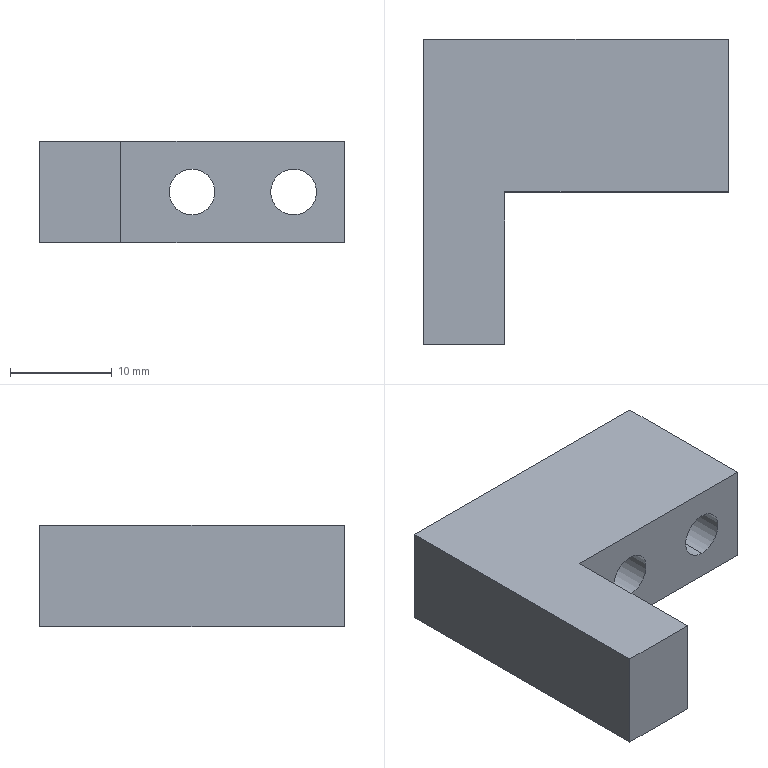Part | STEP file | 227H056244 Stopper_Default | 1 solid | 18 faces | box 30 x 30 x 10 mm | volume 4879 mm3 | plane 10 | cylinder 8 | commonest cylinder face diameters 4.5 x4 8 x4
STEP:
#1=CARTESIAN_POINT('',(0.,0.,0.));
#2=DIRECTION('',(0.,0.,1.));
#3=DIRECTION('',(1.,0.,0.));
#4=AXIS2_PLACEMENT_3D('',#1,#2,#3);
#5=CARTESIAN_POINT('',(10.,10.,4.));
#6=VERTEX_POINT('',#5);
#7=CARTESIAN_POINT('',(10.,15.,4.));
#8=VERTEX_POINT('',#7);
#9=CARTESIAN_POINT('',(10.,15.,4.));
#10=DIRECTION('',(0.,1.,0.));
#11=VECTOR('',#10,1.);
#12=LINE('',#9,#11);
#13=CARTESIAN_POINT('',(10.,15.,0.));
#14=DIRECTION('',(0.,1.,0.));
#15=DIRECTION('',(0.,0.,1.));
#16=AXIS2_PLACEMENT_3D('',#13,#14,#15);
#17=CYLINDRICAL_SURFACE('',#16,4.);
#18=CARTESIAN_POINT('',(6.283,0.));
#19=DIRECTION('',(0.,1.));
#20=VECTOR('',#19,1.);
#21=LINE('',#18,#20);
#22=(GEOMETRIC_REPRESENTATION_CONTEXT(2)PARAMETRIC_REPRESENTATION_CONTEXT()REPRESENTATION_CONTEXT('',''));
#23=DEFINITIONAL_REPRESENTATION('',(#21),#22);
#24=PCURVE('',#17,#23);
#25=CARTESIAN_POINT('',(10.,15.,0.));
#26=DIRECTION('',(0.,1.,0.));
#27=DIRECTION('',(0.,0.,1.));
#28=AXIS2_PLACEMENT_3D('',#25,#26,#27);
#29=CYLINDRICAL_SURFACE('',#28,4.);
#30=CARTESIAN_POINT('',(0.,0.));
#31=DIRECTION('',(0.,1.));
#32=VECTOR('',#31,1.);
#33=LINE('',#30,#32);
#34=(GEOMETRIC_REPRESENTATION_CONTEXT(2)PARAMETRIC_REPRESENTATION_CONTEXT()REPRESENTATION_CONTEXT('',''));
#35=DEFINITIONAL_REPRESENTATION('',(#33),#34);
#36=PCURVE('',#29,#35);
#37=SURFACE_CURVE('',#12,(#24,#36),.PCURVE_S1.);
#38=EDGE_CURVE('',#6,#8,#37,.T.);
#39=ORIENTED_EDGE('',*,*,#38,.T.);
#40=CARTESIAN_POINT('',(10.,15.,-4.));
#41=VERTEX_POINT('',#40);
#42=CARTESIAN_POINT('',(10.,15.,0.));
#43=DIRECTION('',(0.,1.,0.));
#44=DIRECTION('',(0.,0.,1.));
#45=AXIS2_PLACEMENT_3D('',#42,#43,#44);
#46=CIRCLE('',#45,4.);
#47=CARTESIAN_POINT('',(0.,0.));
#48=DIRECTION('',(1.,0.));
#49=VECTOR('',#48,1.);
#50=LINE('',#47,#49);
#51=(GEOMETRIC_REPRESENTATION_CONTEXT(2)PARAMETRIC_REPRESENTATION_CONTEXT()REPRESENTATION_CONTEXT('',''));
#52=DEFINITIONAL_REPRESENTATION('',(#50),#51);
#53=PCURVE('',#17,#52);
#54=CARTESIAN_POINT('',(0.,15.,0.));
#55=DIRECTION('',(0.,1.,0.));
#56=DIRECTION('',(0.,0.,1.));
#57=AXIS2_PLACEMENT_3D('',#54,#55,#56);
#58=PLANE('',#57);
#59=CARTESIAN_POINT('',(0.,10.));
#60=DIRECTION('',(1.,0.));
#61=AXIS2_PLACEMENT_2D('',#59,#60);
#62=CIRCLE('',#61,4.);
#63=(GEOMETRIC_REPRESENTATION_CONTEXT(2)PARAMETRIC_REPRESENTATION_CONTEXT()REPRESENTATION_CONTEXT('',''));
#64=DEFINITIONAL_REPRESENTATION('',(#62),#63);
#65=PCURVE('',#58,#64);
#66=SURFACE_CURVE('',#46,(#53,#65),.PCURVE_S1.);
#67=EDGE_CURVE('',#41,#8,#66,.T.);
#68=ORIENTED_EDGE('',*,*,#67,.F.);
#69=CARTESIAN_POINT('',(10.,10.,-4.));
#70=VERTEX_POINT('',#69);
#71=CARTESIAN_POINT('',(10.,15.,-4.));
#72=DIRECTION('',(0.,1.,0.));
#73=VECTOR('',#72,1.);
#74=LINE('',#71,#73);
#75=CARTESIAN_POINT('',(3.142,0.));
#76=DIRECTION('',(0.,1.));
#77=VECTOR('',#76,1.);
#78=LINE('',#75,#77);
#79=(GEOMETRIC_REPRESENTATION_CONTEXT(2)PARAMETRIC_REPRESENTATION_CONTEXT()REPRESENTATION_CONTEXT('',''));
#80=DEFINITIONAL_REPRESENTATION('',(#78),#79);
#81=PCURVE('',#17,#80);
#82=CARTESIAN_POINT('',(3.142,0.));
#83=DIRECTION('',(0.,1.));
#84=VECTOR('',#83,1.);
#85=LINE('',#82,#84);
#86=(GEOMETRIC_REPRESENTATION_CONTEXT(2)PARAMETRIC_REPRESENTATION_CONTEXT()REPRESENTATION_CONTEXT('',''));
#87=DEFINITIONAL_REPRESENTATION('',(#85),#86);
#88=PCURVE('',#29,#87);
#89=SURFACE_CURVE('',#74,(#81,#88),.PCURVE_S1.);
#90=EDGE_CURVE('',#70,#41,#89,.T.);
#91=ORIENTED_EDGE('',*,*,#90,.F.);
#92=CARTESIAN_POINT('',(10.,10.,0.));
#93=DIRECTION('',(0.,1.,0.));
#94=DIRECTION('',(0.,0.,1.));
#95=AXIS2_PLACEMENT_3D('',#92,#93,#94);
#96=CIRCLE('',#95,4.);
#97=CARTESIAN_POINT('',(0.,-5.));
#98=DIRECTION('',(1.,0.));
#99=VECTOR('',#98,1.);
#100=LINE('',#97,#99);
#101=(GEOMETRIC_REPRESENTATION_CONTEXT(2)PARAMETRIC_REPRESENTATION_CONTEXT()REPRESENTATION_CONTEXT('',''));
#102=DEFINITIONAL_REPRESENTATION('',(#100),#101);
#103=PCURVE('',#17,#102);
#104=CARTESIAN_POINT('',(12.25,10.,0.));
#105=DIRECTION('',(0.,-1.,0.));
#106=DIRECTION('',(0.,0.,-1.));
#107=AXIS2_PLACEMENT_3D('',#104,#105,#106);
#108=PLANE('',#107);
#109=CARTESIAN_POINT('',(-4.,-2.25));
#110=CARTESIAN_POINT('',(-4.,4.678));
#111=CARTESIAN_POINT('',(2.,1.214));
#112=CARTESIAN_POINT('',(8.,-2.25));
#113=CARTESIAN_POINT('',(2.,-5.714));
#114=CARTESIAN_POINT('',(-4.,-9.178));
#115=CARTESIAN_POINT('',(-4.,-2.25));
#116=(BOUNDED_CURVE()B_SPLINE_CURVE(2,(#109,#110,#111,#112,#113,#114,#115),.UNSPECIFIED.,.T.,.F.)B_SPLINE_CURVE_WITH_KNOTS((1,2,2,2,2,1),(-2.094,0.,2.094,4.189,6.283,8.378),.UNSPECIFIED.)CURVE()GEOMETRIC_REPRESENTATION_ITEM()RATIONAL_B_SPLINE_CURVE((1.,0.5,1.,0.5,1.,0.5,1.))REPRESENTATION_ITEM(''));
#117=(GEOMETRIC_REPRESENTATION_CONTEXT(2)PARAMETRIC_REPRESENTATION_CONTEXT()REPRESENTATION_CONTEXT('',''));
#118=DEFINITIONAL_REPRESENTATION('',(#116),#117);
#119=PCURVE('',#108,#118);
#120=SURFACE_CURVE('',#96,(#103,#119),.PCURVE_S1.);
#121=EDGE_CURVE('',#70,#6,#120,.T.);
#122=ORIENTED_EDGE('',*,*,#121,.T.);
#123=EDGE_LOOP('',(#39,#68,#91,#122));
#124=FACE_BOUND('',#123,.F.);
#125=ADVANCED_FACE('',(#124),#17,.F.);
#126=CARTESIAN_POINT('',(10.,0.,2.25));
#127=VERTEX_POINT('',#126);
#128=CARTESIAN_POINT('',(10.,10.,2.25));
#129=VERTEX_POINT('',#128);
#130=CARTESIAN_POINT('',(10.,15.,2.25));
#131=DIRECTION('',(0.,1.,0.));
#132=VECTOR('',#131,1.);
#133=LINE('',#130,#132);
#134=CARTESIAN_POINT('',(10.,15.,0.));
#135=DIRECTION('',(0.,1.,0.));
#136=DIRECTION('',(0.,0.,1.));
#137=AXIS2_PLACEMENT_3D('',#134,#135,#136);
#138=CYLINDRICAL_SURFACE('',#137,2.25);
#139=CARTESIAN_POINT('',(6.283,0.));
#140=DIRECTION('',(0.,1.));
#141=VECTOR('',#140,1.);
#142=LINE('',#139,#141);
#143=(GEOMETRIC_REPRESENTATION_CONTEXT(2)PARAMETRIC_REPRESENTATION_CONTEXT()REPRESENTATION_CONTEXT('',''));
#144=DEFINITIONAL_REPRESENTATION('',(#142),#143);
#145=PCURVE('',#138,#144);
#146=CARTESIAN_POINT('',(10.,15.,0.));
#147=DIRECTION('',(0.,1.,0.));
#148=DIRECTION('',(0.,0.,1.));
#149=AXIS2_PLACEMENT_3D('',#146,#147,#148);
#150=CYLINDRICAL_SURFACE('',#149,2.25);
#151=CARTESIAN_POINT('',(0.,0.));
#152=DIRECTION('',(0.,1.));
#153=VECTOR('',#152,1.);
#154=LINE('',#151,#153);
#155=(GEOMETRIC_REPRESENTATION_CONTEXT(2)PARAMETRIC_REPRESENTATION_CONTEXT()REPRESENTATION_CONTEXT('',''));
#156=DEFINITIONAL_REPRESENTATION('',(#154),#155);
#157=PCURVE('',#150,#156);
#158=SURFACE_CURVE('',#133,(#145,#157),.PCURVE_S1.);
#159=EDGE_CURVE('',#127,#129,#158,.T.);
#160=ORIENTED_EDGE('',*,*,#159,.T.);
#161=CARTESIAN_POINT('',(10.,10.,-2.25));
#162=VERTEX_POINT('',#161);
#163=CARTESIAN_POINT('',(10.,10.,0.));
#164=DIRECTION('',(0.,1.,0.));
#165=DIRECTION('',(0.,0.,1.));
#166=AXIS2_PLACEMENT_3D('',#163,#164,#165);
#167=CIRCLE('',#166,2.25);
#168=CARTESIAN_POINT('',(0.,-5.));
#169=DIRECTION('',(1.,0.));
#170=VECTOR('',#169,1.);
#171=LINE('',#168,#170);
#172=(GEOMETRIC_REPRESENTATION_CONTEXT(2)PARAMETRIC_REPRESENTATION_CONTEXT()REPRESENTATION_CONTEXT('',''));
#173=DEFINITIONAL_REPRESENTATION('',(#171),#172);
#174=PCURVE('',#138,#173);
#175=CARTESIAN_POINT('',(-2.25,-2.25));
#176=CARTESIAN_POINT('',(-2.25,1.647));
#177=CARTESIAN_POINT('',(1.125,-0.3014));
#178=CARTESIAN_POINT('',(4.5,-2.25));
#179=CARTESIAN_POINT('',(1.125,-4.199));
#180=CARTESIAN_POINT('',(-2.25,-6.147));
#181=CARTESIAN_POINT('',(-2.25,-2.25));
#182=(BOUNDED_CURVE()B_SPLINE_CURVE(2,(#175,#176,#177,#178,#179,#180,#181),.UNSPECIFIED.,.T.,.F.)B_SPLINE_CURVE_WITH_KNOTS((1,2,2,2,2,1),(-2.094,0.,2.094,4.189,6.283,8.378),.UNSPECIFIED.)CURVE()GEOMETRIC_REPRESENTATION_ITEM()RATIONAL_B_SPLINE_CURVE((1.,0.5,1.,0.5,1.,0.5,1.))REPRESENTATION_ITEM(''));
#183=(GEOMETRIC_REPRESENTATION_CONTEXT(2)PARAMETRIC_REPRESENTATION_CONTEXT()REPRESENTATION_CONTEXT('',''));
#184=DEFINITIONAL_REPRESENTATION('',(#182),#183);
#185=PCURVE('',#108,#184);
#186=SURFACE_CURVE('',#167,(#174,#185),.PCURVE_S1.);
#187=EDGE_CURVE('',#162,#129,#186,.T.);
#188=ORIENTED_EDGE('',*,*,#187,.F.);
#189=CARTESIAN_POINT('',(10.,0.,-2.25));
#190=VERTEX_POINT('',#189);
#191=CARTESIAN_POINT('',(10.,15.,-2.25));
#192=DIRECTION('',(0.,1.,0.));
#193=VECTOR('',#192,1.);
#194=LINE('',#191,#193);
#195=CARTESIAN_POINT('',(3.142,0.));
#196=DIRECTION('',(0.,1.));
#197=VECTOR('',#196,1.);
#198=LINE('',#195,#197);
#199=(GEOMETRIC_REPRESENTATION_CONTEXT(2)PARAMETRIC_REPRESENTATION_CONTEXT()REPRESENTATION_CONTEXT('',''));
#200=DEFINITIONAL_REPRESENTATION('',(#198),#199);
#201=PCURVE('',#138,#200);
#202=CARTESIAN_POINT('',(3.142,0.));
#203=DIRECTION('',(0.,1.));
#204=VECTOR('',#203,1.);
#205=LINE('',#202,#204);
#206=(GEOMETRIC_REPRESENTATION_CONTEXT(2)PARAMETRIC_REPRESENTATION_CONTEXT()REPRESENTATION_CONTEXT('',''));
#207=DEFINITIONAL_REPRESENTATION('',(#205),#206);
#208=PCURVE('',#150,#207);
#209=SURFACE_CURVE('',#194,(#201,#208),.PCURVE_S1.);
#210=EDGE_CURVE('',#190,#162,#209,.T.);
#211=ORIENTED_EDGE('',*,*,#210,.F.);
#212=CARTESIAN_POINT('',(10.,0.,0.));
#213=DIRECTION('',(0.,1.,0.));
#214=DIRECTION('',(0.,0.,1.));
#215=AXIS2_PLACEMENT_3D('',#212,#213,#214);
#216=CIRCLE('',#215,2.25);
#217=CARTESIAN_POINT('',(0.,-15.));
#218=DIRECTION('',(1.,0.));
#219=VECTOR('',#218,1.);
#220=LINE('',#217,#219);
#221=(GEOMETRIC_REPRESENTATION_CONTEXT(2)PARAMETRIC_REPRESENTATION_CONTEXT()REPRESENTATION_CONTEXT('',''));
#222=DEFINITIONAL_REPRESENTATION('',(#220),#221);
#223=PCURVE('',#138,#222);
#224=CARTESIAN_POINT('',(0.,0.,0.));
#225=DIRECTION('',(0.,1.,0.));
#226=DIRECTION('',(0.,0.,1.));
#227=AXIS2_PLACEMENT_3D('',#224,#225,#226);
#228=PLANE('',#227);
#229=CARTESIAN_POINT('',(0.,10.));
#230=DIRECTION('',(1.,0.));
#231=AXIS2_PLACEMENT_2D('',#229,#230);
#232=CIRCLE('',#231,2.25);
#233=(GEOMETRIC_REPRESENTATION_CONTEXT(2)PARAMETRIC_REPRESENTATION_CONTEXT()REPRESENTATION_CONTEXT('',''));
#234=DEFINITIONAL_REPRESENTATION('',(#232),#233);
#235=PCURVE('',#228,#234);
#236=SURFACE_CURVE('',#216,(#223,#235),.PCURVE_S1.);
#237=EDGE_CURVE('',#190,#127,#236,.T.);
#238=ORIENTED_EDGE('',*,*,#237,.T.);
#239=EDGE_LOOP('',(#160,#188,#211,#238));
#240=FACE_BOUND('',#239,.F.);
#241=ADVANCED_FACE('',(#240),#138,.F.);
#242=CARTESIAN_POINT('',(0.,10.,4.));
#243=VERTEX_POINT('',#242);
#244=CARTESIAN_POINT('',(0.,15.,4.));
#245=VERTEX_POINT('',#244);
#246=CARTESIAN_POINT('',(0.,15.,4.));
#247=DIRECTION('',(0.,1.,0.));
#248=VECTOR('',#247,1.);
#249=LINE('',#246,#248);
#250=CARTESIAN_POINT('',(0.,15.,0.));
#251=DIRECTION('',(0.,1.,0.));
#252=DIRECTION('',(0.,0.,1.));
#253=AXIS2_PLACEMENT_3D('',#250,#251,#252);
#254=CYLINDRICAL_SURFACE('',#253,4.);
#255=CARTESIAN_POINT('',(6.283,0.));
#256=DIRECTION('',(0.,1.));
#257=VECTOR('',#256,1.);
#258=LINE('',#255,#257);
#259=(GEOMETRIC_REPRESENTATION_CONTEXT(2)PARAMETRIC_REPRESENTATION_CONTEXT()REPRESENTATION_CONTEXT('',''));
#260=DEFINITIONAL_REPRESENTATION('',(#258),#259);
#261=PCURVE('',#254,#260);
#262=CARTESIAN_POINT('',(0.,15.,0.));
#263=DIRECTION('',(0.,1.,0.));
#264=DIRECTION('',(0.,0.,1.));
#265=AXIS2_PLACEMENT_3D('',#262,#263,#264);
#266=CYLINDRICAL_SURFACE('',#265,4.);
#267=CARTESIAN_POINT('',(0.,0.));
#268=DIRECTION('',(0.,1.));
#269=VECTOR('',#268,1.);
#270=LINE('',#267,#269);
#271=(GEOMETRIC_REPRESENTATION_CONTEXT(2)PARAMETRIC_REPRESENTATION_CONTEXT()REPRESENTATION_CONTEXT('',''));
#272=DEFINITIONAL_REPRESENTATION('',(#270),#271);
#273=PCURVE('',#266,#272);
#274=SURFACE_CURVE('',#249,(#261,#273),.PCURVE_S1.);
#275=EDGE_CURVE('',#243,#245,#274,.T.);
#276=ORIENTED_EDGE('',*,*,#275,.T.);
#277=CARTESIAN_POINT('',(0.,15.,-4.));
#278=VERTEX_POINT('',#277);
#279=CARTESIAN_POINT('',(0.,15.,0.));
#280=DIRECTION('',(0.,1.,0.));
#281=DIRECTION('',(0.,0.,1.));
#282=AXIS2_PLACEMENT_3D('',#279,#280,#281);
#283=CIRCLE('',#282,4.);
#284=CARTESIAN_POINT('',(0.,0.));
#285=DIRECTION('',(1.,0.));
#286=VECTOR('',#285,1.);
#287=LINE('',#284,#286);
#288=(GEOMETRIC_REPRESENTATION_CONTEXT(2)PARAMETRIC_REPRESENTATION_CONTEXT()REPRESENTATION_CONTEXT('',''));
#289=DEFINITIONAL_REPRESENTATION('',(#287),#288);
#290=PCURVE('',#254,#289);
#291=CARTESIAN_POINT('',(0.,0.));
#292=DIRECTION('',(1.,0.));
#293=AXIS2_PLACEMENT_2D('',#291,#292);
#294=CIRCLE('',#293,4.);
#295=(GEOMETRIC_REPRESENTATION_CONTEXT(2)PARAMETRIC_REPRESENTATION_CONTEXT()REPRESENTATION_CONTEXT('',''));
#296=DEFINITIONAL_REPRESENTATION('',(#294),#295);
#297=PCURVE('',#58,#296);
#298=SURFACE_CURVE('',#283,(#290,#297),.PCURVE_S1.);
#299=EDGE_CURVE('',#278,#245,#298,.T.);
#300=ORIENTED_EDGE('',*,*,#299,.F.);
#301=CARTESIAN_POINT('',(0.,10.,-4.));
#302=VERTEX_POINT('',#301);
#303=CARTESIAN_POINT('',(0.,15.,-4.));
#304=DIRECTION('',(0.,1.,0.));
#305=VECTOR('',#304,1.);
#306=LINE('',#303,#305);
#307=CARTESIAN_POINT('',(3.142,0.));
#308=DIRECTION('',(0.,1.));
#309=VECTOR('',#308,1.);
#310=LINE('',#307,#309);
#311=(GEOMETRIC_REPRESENTATION_CONTEXT(2)PARAMETRIC_REPRESENTATION_CONTEXT()REPRESENTATION_CONTEXT('',''));
#312=DEFINITIONAL_REPRESENTATION('',(#310),#311);
#313=PCURVE('',#254,#312);
#314=CARTESIAN_POINT('',(3.142,0.));
#315=DIRECTION('',(0.,1.));
#316=VECTOR('',#315,1.);
#317=LINE('',#314,#316);
#318=(GEOMETRIC_REPRESENTATION_CONTEXT(2)PARAMETRIC_REPRESENTATION_CONTEXT()REPRESENTATION_CONTEXT('',''));
#319=DEFINITIONAL_REPRESENTATION('',(#317),#318);
#320=PCURVE('',#266,#319);
#321=SURFACE_CURVE('',#306,(#313,#320),.PCURVE_S1.);
#322=EDGE_CURVE('',#302,#278,#321,.T.);
#323=ORIENTED_EDGE('',*,*,#322,.F.);
#324=CARTESIAN_POINT('',(0.,10.,0.));
#325=DIRECTION('',(0.,1.,0.));
#326=DIRECTION('',(0.,0.,1.));
#327=AXIS2_PLACEMENT_3D('',#324,#325,#326);
#328=CIRCLE('',#327,4.);
#329=CARTESIAN_POINT('',(0.,-5.));
#330=DIRECTION('',(1.,0.));
#331=VECTOR('',#330,1.);
#332=LINE('',#329,#331);
#333=(GEOMETRIC_REPRESENTATION_CONTEXT(2)PARAMETRIC_REPRESENTATION_CONTEXT()REPRESENTATION_CONTEXT('',''));
#334=DEFINITIONAL_REPRESENTATION('',(#332),#333);
#335=PCURVE('',#254,#334);
#336=CARTESIAN_POINT('',(2.25,10.,0.));
#337=DIRECTION('',(0.,-1.,0.));
#338=DIRECTION('',(0.,0.,-1.));
#339=AXIS2_PLACEMENT_3D('',#336,#337,#338);
#340=PLANE('',#339);
#341=CARTESIAN_POINT('',(-4.,-2.25));
#342=CARTESIAN_POINT('',(-4.,4.678));
#343=CARTESIAN_POINT('',(2.,1.214));
#344=CARTESIAN_POINT('',(8.,-2.25));
#345=CARTESIAN_POINT('',(2.,-5.714));
#346=CARTESIAN_POINT('',(-4.,-9.178));
#347=CARTESIAN_POINT('',(-4.,-2.25));
#348=(BOUNDED_CURVE()B_SPLINE_CURVE(2,(#341,#342,#343,#344,#345,#346,#347),.UNSPECIFIED.,.T.,.F.)B_SPLINE_CURVE_WITH_KNOTS((1,2,2,2,2,1),(-2.094,0.,2.094,4.189,6.283,8.378),.UNSPECIFIED.)CURVE()GEOMETRIC_REPRESENTATION_ITEM()RATIONAL_B_SPLINE_CURVE((1.,0.5,1.,0.5,1.,0.5,1.))REPRESENTATION_ITEM(''));
#349=(GEOMETRIC_REPRESENTATION_CONTEXT(2)PARAMETRIC_REPRESENTATION_CONTEXT()REPRESENTATION_CONTEXT('',''));
#350=DEFINITIONAL_REPRESENTATION('',(#348),#349);
#351=PCURVE('',#340,#350);
#352=SURFACE_CURVE('',#328,(#335,#351),.PCURVE_S1.);
#353=EDGE_CURVE('',#302,#243,#352,.T.);
#354=ORIENTED_EDGE('',*,*,#353,.T.);
#355=EDGE_LOOP('',(#276,#300,#323,#354));
#356=FACE_BOUND('',#355,.F.);
#357=ADVANCED_FACE('',(#356),#254,.F.);
#358=CARTESIAN_POINT('',(0.,0.,2.25));
#359=VERTEX_POINT('',#358);
#360=CARTESIAN_POINT('',(0.,10.,2.25));
#361=VERTEX_POINT('',#360);
#362=CARTESIAN_POINT('',(0.,15.,2.25));
#363=DIRECTION('',(0.,1.,0.));
#364=VECTOR('',#363,1.);
#365=LINE('',#362,#364);
#366=CARTESIAN_POINT('',(0.,15.,0.));
#367=DIRECTION('',(0.,1.,0.));
#368=DIRECTION('',(0.,0.,1.));
#369=AXIS2_PLACEMENT_3D('',#366,#367,#368);
#370=CYLINDRICAL_SURFACE('',#369,2.25);
#371=CARTESIAN_POINT('',(6.283,0.));
#372=DIRECTION('',(0.,1.));
#373=VECTOR('',#372,1.);
#374=LINE('',#371,#373);
#375=(GEOMETRIC_REPRESENTATION_CONTEXT(2)PARAMETRIC_REPRESENTATION_CONTEXT()REPRESENTATION_CONTEXT('',''));
#376=DEFINITIONAL_REPRESENTATION('',(#374),#375);
#377=PCURVE('',#370,#376);
#378=CARTESIAN_POINT('',(0.,15.,0.));
#379=DIRECTION('',(0.,1.,0.));
#380=DIRECTION('',(0.,0.,1.));
#381=AXIS2_PLACEMENT_3D('',#378,#379,#380);
#382=CYLINDRICAL_SURFACE('',#381,2.25);
#383=CARTESIAN_POINT('',(0.,0.));
#384=DIRECTION('',(0.,1.));
#385=VECTOR('',#384,1.);
#386=LINE('',#383,#385);
#387=(GEOMETRIC_REPRESENTATION_CONTEXT(2)PARAMETRIC_REPRESENTATION_CONTEXT()REPRESENTATION_CONTEXT('',''));
#388=DEFINITIONAL_REPRESENTATION('',(#386),#387);
#389=PCURVE('',#382,#388);
#390=SURFACE_CURVE('',#365,(#377,#389),.PCURVE_S1.);
#391=EDGE_CURVE('',#359,#361,#390,.T.);
#392=ORIENTED_EDGE('',*,*,#391,.T.);
#393=CARTESIAN_POINT('',(0.,10.,-2.25));
#394=VERTEX_POINT('',#393);
#395=CARTESIAN_POINT('',(0.,10.,0.));
#396=DIRECTION('',(0.,1.,0.));
#397=DIRECTION('',(0.,0.,1.));
#398=AXIS2_PLACEMENT_3D('',#395,#396,#397);
#399=CIRCLE('',#398,2.25);
#400=CARTESIAN_POINT('',(0.,-5.));
#401=DIRECTION('',(1.,0.));
#402=VECTOR('',#401,1.);
#403=LINE('',#400,#402);
#404=(GEOMETRIC_REPRESENTATION_CONTEXT(2)PARAMETRIC_REPRESENTATION_CONTEXT()REPRESENTATION_CONTEXT('',''));
#405=DEFINITIONAL_REPRESENTATION('',(#403),#404);
#406=PCURVE('',#370,#405);
#407=CARTESIAN_POINT('',(-2.25,-2.25));
#408=CARTESIAN_POINT('',(-2.25,1.647));
#409=CARTESIAN_POINT('',(1.125,-0.3014));
#410=CARTESIAN_POINT('',(4.5,-2.25));
#411=CARTESIAN_POINT('',(1.125,-4.199));
#412=CARTESIAN_POINT('',(-2.25,-6.147));
#413=CARTESIAN_POINT('',(-2.25,-2.25));
#414=(BOUNDED_CURVE()B_SPLINE_CURVE(2,(#407,#408,#409,#410,#411,#412,#413),.UNSPECIFIED.,.T.,.F.)B_SPLINE_CURVE_WITH_KNOTS((1,2,2,2,2,1),(-2.094,0.,2.094,4.189,6.283,8.378),.UNSPECIFIED.)CURVE()GEOMETRIC_REPRESENTATION_ITEM()RATIONAL_B_SPLINE_CURVE((1.,0.5,1.,0.5,1.,0.5,1.))REPRESENTATION_ITEM(''));
#415=(GEOMETRIC_REPRESENTATION_CONTEXT(2)PARAMETRIC_REPRESENTATION_CONTEXT()REPRESENTATION_CONTEXT('',''));
#416=DEFINITIONAL_REPRESENTATION('',(#414),#415);
#417=PCURVE('',#340,#416);
#418=SURFACE_CURVE('',#399,(#406,#417),.PCURVE_S1.);
#419=EDGE_CURVE('',#394,#361,#418,.T.);
#420=ORIENTED_EDGE('',*,*,#419,.F.);
#421=CARTESIAN_POINT('',(0.,0.,-2.25));
#422=VERTEX_POINT('',#421);
#423=CARTESIAN_POINT('',(0.,15.,-2.25));
#424=DIRECTION('',(0.,1.,0.));
#425=VECTOR('',#424,1.);
#426=LINE('',#423,#425);
#427=CARTESIAN_POINT('',(3.142,0.));
#428=DIRECTION('',(0.,1.));
#429=VECTOR('',#428,1.);
#430=LINE('',#427,#429);
#431=(GEOMETRIC_REPRESENTATION_CONTEXT(2)PARAMETRIC_REPRESENTATION_CONTEXT()REPRESENTATION_CONTEXT('',''));
#432=DEFINITIONAL_REPRESENTATION('',(#430),#431);
#433=PCURVE('',#370,#432);
#434=CARTESIAN_POINT('',(3.142,0.));
#435=DIRECTION('',(0.,1.));
#436=VECTOR('',#435,1.);
#437=LINE('',#434,#436);
#438=(GEOMETRIC_REPRESENTATION_CONTEXT(2)PARAMETRIC_REPRESENTATION_CONTEXT()REPRESENTATION_CONTEXT('',''));
#439=DEFINITIONAL_REPRESENTATION('',(#437),#438);
#440=PCURVE('',#382,#439);
#441=SURFACE_CURVE('',#426,(#433,#440),.PCURVE_S1.);
#442=EDGE_CURVE('',#422,#394,#441,.T.);
#443=ORIENTED_EDGE('',*,*,#442,.F.);
#444=CARTESIAN_POINT('',(0.,0.,0.));
#445=DIRECTION('',(0.,1.,0.));
#446=DIRECTION('',(0.,0.,1.));
#447=AXIS2_PLACEMENT_3D('',#444,#445,#446);
#448=CIRCLE('',#447,2.25);
#449=CARTESIAN_POINT('',(0.,-15.));
#450=DIRECTION('',(1.,0.));
#451=VECTOR('',#450,1.);
#452=LINE('',#449,#451);
#453=(GEOMETRIC_REPRESENTATION_CONTEXT(2)PARAMETRIC_REPRESENTATION_CONTEXT()REPRESENTATION_CONTEXT('',''));
#454=DEFINITIONAL_REPRESENTATION('',(#452),#453);
#455=PCURVE('',#370,#454);
#456=CARTESIAN_POINT('',(0.,0.));
#457=DIRECTION('',(1.,0.));
#458=AXIS2_PLACEMENT_2D('',#456,#457);
#459=CIRCLE('',#458,2.25);
#460=(GEOMETRIC_REPRESENTATION_CONTEXT(2)PARAMETRIC_REPRESENTATION_CONTEXT()REPRESENTATION_CONTEXT('',''));
#461=DEFINITIONAL_REPRESENTATION('',(#459),#460);
#462=PCURVE('',#228,#461);
#463=SURFACE_CURVE('',#448,(#455,#462),.PCURVE_S1.);
#464=EDGE_CURVE('',#422,#359,#463,.T.);
#465=ORIENTED_EDGE('',*,*,#464,.T.);
#466=EDGE_LOOP('',(#392,#420,#443,#465));
#467=FACE_BOUND('',#466,.F.);
#468=ADVANCED_FACE('',(#467),#370,.F.);
#469=CARTESIAN_POINT('',(-15.,15.,-5.));
#470=VERTEX_POINT('',#469);
#471=CARTESIAN_POINT('',(-15.,-15.,-5.));
#472=VERTEX_POINT('',#471);
#473=CARTESIAN_POINT('',(-15.,15.,-5.));
#474=DIRECTION('',(0.,-1.,0.));
#475=VECTOR('',#474,1.);
#476=LINE('',#473,#475);
#477=CARTESIAN_POINT('',(-15.,15.,5.));
#478=DIRECTION('',(1.,0.,0.));
#479=DIRECTION('',(0.,0.,-1.));
#480=AXIS2_PLACEMENT_3D('',#477,#478,#479);
#481=PLANE('',#480);
#482=CARTESIAN_POINT('',(10.,0.));
#483=DIRECTION('',(0.,-1.));
#484=VECTOR('',#483,1.);
#485=LINE('',#482,#484);
#486=(GEOMETRIC_REPRESENTATION_CONTEXT(2)PARAMETRIC_REPRESENTATION_CONTEXT()REPRESENTATION_CONTEXT('',''));
#487=DEFINITIONAL_REPRESENTATION('',(#485),#486);
#488=PCURVE('',#481,#487);
#489=CARTESIAN_POINT('',(15.,15.,-5.));
#490=DIRECTION('',(0.,0.,1.));
#491=DIRECTION('',(1.,0.,0.));
#492=AXIS2_PLACEMENT_3D('',#489,#490,#491);
#493=PLANE('',#492);
#494=CARTESIAN_POINT('',(-30.,0.));
#495=DIRECTION('',(0.,-1.));
#496=VECTOR('',#495,1.);
#497=LINE('',#494,#496);
#498=(GEOMETRIC_REPRESENTATION_CONTEXT(2)PARAMETRIC_REPRESENTATION_CONTEXT()REPRESENTATION_CONTEXT('',''));
#499=DEFINITIONAL_REPRESENTATION('',(#497),#498);
#500=PCURVE('',#493,#499);
#501=SURFACE_CURVE('',#476,(#488,#500),.PCURVE_S1.);
#502=EDGE_CURVE('',#470,#472,#501,.T.);
#503=ORIENTED_EDGE('',*,*,#502,.T.);
#504=CARTESIAN_POINT('',(-15.,-15.,5.));
#505=VERTEX_POINT('',#504);
#506=CARTESIAN_POINT('',(-15.,-15.,22.));
#507=DIRECTION('',(0.,0.,-1.));
#508=VECTOR('',#507,1.);
#509=LINE('',#506,#508);
#510=CARTESIAN_POINT('',(-17.,-30.));
#511=DIRECTION('',(1.,0.));
#512=VECTOR('',#511,1.);
#513=LINE('',#510,#512);
#514=(GEOMETRIC_REPRESENTATION_CONTEXT(2)PARAMETRIC_REPRESENTATION_CONTEXT()REPRESENTATION_CONTEXT('',''));
#515=DEFINITIONAL_REPRESENTATION('',(#513),#514);
#516=PCURVE('',#481,#515);
#517=CARTESIAN_POINT('',(-15.,-15.,22.));
#518=DIRECTION('',(0.,-1.,0.));
#519=DIRECTION('',(0.,0.,-1.));
#520=AXIS2_PLACEMENT_3D('',#517,#518,#519);
#521=PLANE('',#520);
#522=CARTESIAN_POINT('',(0.,0.));
#523=DIRECTION('',(1.,0.));
#524=VECTOR('',#523,1.);
#525=LINE('',#522,#524);
#526=(GEOMETRIC_REPRESENTATION_CONTEXT(2)PARAMETRIC_REPRESENTATION_CONTEXT()REPRESENTATION_CONTEXT('',''));
#527=DEFINITIONAL_REPRESENTATION('',(#525),#526);
#528=PCURVE('',#521,#527);
#529=SURFACE_CURVE('',#509,(#516,#528),.PCURVE_S1.);
#530=EDGE_CURVE('',#505,#472,#529,.T.);
#531=ORIENTED_EDGE('',*,*,#530,.F.);
#532=CARTESIAN_POINT('',(-15.,15.,5.));
#533=VERTEX_POINT('',#532);
#534=CARTESIAN_POINT('',(-15.,15.,5.));
#535=DIRECTION('',(0.,-1.,0.));
#536=VECTOR('',#535,1.);
#537=LINE('',#534,#536);
#538=CARTESIAN_POINT('',(0.,0.));
#539=DIRECTION('',(0.,-1.));
#540=VECTOR('',#539,1.);
#541=LINE('',#538,#540);
#542=(GEOMETRIC_REPRESENTATION_CONTEXT(2)PARAMETRIC_REPRESENTATION_CONTEXT()REPRESENTATION_CONTEXT('',''));
#543=DEFINITIONAL_REPRESENTATION('',(#541),#542);
#544=PCURVE('',#481,#543);
#545=CARTESIAN_POINT('',(15.,15.,5.));
#546=DIRECTION('',(0.,0.,-1.));
#547=DIRECTION('',(-1.,0.,0.));
#548=AXIS2_PLACEMENT_3D('',#545,#546,#547);
#549=PLANE('',#548);
#550=CARTESIAN_POINT('',(30.,0.));
#551=DIRECTION('',(0.,-1.));
#552=VECTOR('',#551,1.);
#553=LINE('',#550,#552);
#554=(GEOMETRIC_REPRESENTATION_CONTEXT(2)PARAMETRIC_REPRESENTATION_CONTEXT()REPRESENTATION_CONTEXT('',''));
#555=DEFINITIONAL_REPRESENTATION('',(#553),#554);
#556=PCURVE('',#549,#555);
#557=SURFACE_CURVE('',#537,(#544,#556),.PCURVE_S1.);
#558=EDGE_CURVE('',#533,#505,#557,.T.);
#559=ORIENTED_EDGE('',*,*,#558,.F.);
#560=CARTESIAN_POINT('',(-15.,15.,5.));
#561=DIRECTION('',(0.,0.,1.));
#562=VECTOR('',#561,1.);
#563=LINE('',#560,#562);
#564=CARTESIAN_POINT('',(0.,0.));
#565=DIRECTION('',(-1.,0.));
#566=VECTOR('',#565,1.);
#567=LINE('',#564,#566);
#568=(GEOMETRIC_REPRESENTATION_CONTEXT(2)PARAMETRIC_REPRESENTATION_CONTEXT()REPRESENTATION_CONTEXT('',''));
#569=DEFINITIONAL_REPRESENTATION('',(#567),#568);
#570=PCURVE('',#481,#569);
#571=CARTESIAN_POINT('',(5.,-15.));
#572=DIRECTION('',(1.,0.));
#573=VECTOR('',#572,1.);
#574=LINE('',#571,#573);
#575=(GEOMETRIC_REPRESENTATION_CONTEXT(2)PARAMETRIC_REPRESENTATION_CONTEXT()REPRESENTATION_CONTEXT('',''));
#576=DEFINITIONAL_REPRESENTATION('',(#574),#575);
#577=PCURVE('',#58,#576);
#578=SURFACE_CURVE('',#563,(#570,#577),.PCURVE_S1.);
#579=EDGE_CURVE('',#470,#533,#578,.T.);
#580=ORIENTED_EDGE('',*,*,#579,.F.);
#581=EDGE_LOOP('',(#503,#531,#559,#580));
#582=FACE_BOUND('',#581,.T.);
#583=ADVANCED_FACE('',(#582),#481,.F.);
#584=ORIENTED_EDGE('',*,*,#558,.T.);
#585=CARTESIAN_POINT('',(-7.,-15.,5.));
#586=VERTEX_POINT('',#585);
#587=CARTESIAN_POINT('',(-15.,-15.,5.));
#588=DIRECTION('',(1.,0.,0.));
#589=VECTOR('',#588,1.);
#590=LINE('',#587,#589);
#591=CARTESIAN_POINT('',(30.,-30.));
#592=DIRECTION('',(-1.,0.));
#593=VECTOR('',#592,1.);
#594=LINE('',#591,#593);
#595=(GEOMETRIC_REPRESENTATION_CONTEXT(2)PARAMETRIC_REPRESENTATION_CONTEXT()REPRESENTATION_CONTEXT('',''));
#596=DEFINITIONAL_REPRESENTATION('',(#594),#595);
#597=PCURVE('',#549,#596);
#598=CARTESIAN_POINT('',(17.,0.));
#599=DIRECTION('',(0.,1.));
#600=VECTOR('',#599,1.);
#601=LINE('',#598,#600);
#602=(GEOMETRIC_REPRESENTATION_CONTEXT(2)PARAMETRIC_REPRESENTATION_CONTEXT()REPRESENTATION_CONTEXT('',''));
#603=DEFINITIONAL_REPRESENTATION('',(#601),#602);
#604=PCURVE('',#521,#603);
#605=SURFACE_CURVE('',#590,(#597,#604),.PCURVE_S1.);
#606=EDGE_CURVE('',#505,#586,#605,.T.);
#607=ORIENTED_EDGE('',*,*,#606,.T.);
#608=CARTESIAN_POINT('',(-7.,0.,5.));
#609=VERTEX_POINT('',#608);
#610=CARTESIAN_POINT('',(-7.,0.,5.));
#611=DIRECTION('',(0.,1.,0.));
#612=VECTOR('',#611,1.);
#613=LINE('',#610,#612);
#614=CARTESIAN_POINT('',(22.,-15.));
#615=DIRECTION('',(0.,1.));
#616=VECTOR('',#615,1.);
#617=LINE('',#614,#616);
#618=(GEOMETRIC_REPRESENTATION_CONTEXT(2)PARAMETRIC_REPRESENTATION_CONTEXT()REPRESENTATION_CONTEXT('',''));
#619=DEFINITIONAL_REPRESENTATION('',(#617),#618);
#620=PCURVE('',#549,#619);
#621=CARTESIAN_POINT('',(-7.,0.,22.));
#622=DIRECTION('',(1.,0.,0.));
#623=DIRECTION('',(0.,1.,0.));
#624=AXIS2_PLACEMENT_3D('',#621,#622,#623);
#625=PLANE('',#624);
#626=CARTESIAN_POINT('',(0.,-17.));
#627=DIRECTION('',(1.,0.));
#628=VECTOR('',#627,1.);
#629=LINE('',#626,#628);
#630=(GEOMETRIC_REPRESENTATION_CONTEXT(2)PARAMETRIC_REPRESENTATION_CONTEXT()REPRESENTATION_CONTEXT('',''));
#631=DEFINITIONAL_REPRESENTATION('',(#629),#630);
#632=PCURVE('',#625,#631);
#633=SURFACE_CURVE('',#613,(#620,#632),.PCURVE_S1.);
#634=EDGE_CURVE('',#586,#609,#633,.T.);
#635=ORIENTED_EDGE('',*,*,#634,.T.);
#636=CARTESIAN_POINT('',(15.,0.,5.));
#637=VERTEX_POINT('',#636);
#638=CARTESIAN_POINT('',(15.,0.,5.));
#639=DIRECTION('',(1.,0.,0.));
#640=VECTOR('',#639,1.);
#641=LINE('',#638,#640);
#642=CARTESIAN_POINT('',(0.,-15.));
#643=DIRECTION('',(-1.,0.));
#644=VECTOR('',#643,1.);
#645=LINE('',#642,#644);
#646=(GEOMETRIC_REPRESENTATION_CONTEXT(2)PARAMETRIC_REPRESENTATION_CONTEXT()REPRESENTATION_CONTEXT('',''));
#647=DEFINITIONAL_REPRESENTATION('',(#645),#646);
#648=PCURVE('',#549,#647);
#649=CARTESIAN_POINT('',(5.,15.));
#650=DIRECTION('',(0.,1.));
#651=VECTOR('',#650,1.);
#652=LINE('',#649,#651);
#653=(GEOMETRIC_REPRESENTATION_CONTEXT(2)PARAMETRIC_REPRESENTATION_CONTEXT()REPRESENTATION_CONTEXT('',''));
#654=DEFINITIONAL_REPRESENTATION('',(#652),#653);
#655=PCURVE('',#228,#654);
#656=SURFACE_CURVE('',#641,(#648,#655),.PCURVE_S1.);
#657=EDGE_CURVE('',#609,#637,#656,.T.);
#658=ORIENTED_EDGE('',*,*,#657,.T.);
#659=CARTESIAN_POINT('',(15.,15.,5.));
#660=VERTEX_POINT('',#659);
#661=CARTESIAN_POINT('',(15.,15.,5.));
#662=DIRECTION('',(0.,-1.,0.));
#663=VECTOR('',#662,1.);
#664=LINE('',#661,#663);
#665=CARTESIAN_POINT('',(0.,0.));
#666=DIRECTION('',(0.,-1.));
#667=VECTOR('',#666,1.);
#668=LINE('',#665,#667);
#669=(GEOMETRIC_REPRESENTATION_CONTEXT(2)PARAMETRIC_REPRESENTATION_CONTEXT()REPRESENTATION_CONTEXT('',''));
#670=DEFINITIONAL_REPRESENTATION('',(#668),#669);
#671=PCURVE('',#549,#670);
#672=CARTESIAN_POINT('',(15.,15.,5.));
#673=DIRECTION('',(-1.,0.,0.));
#674=DIRECTION('',(0.,0.,1.));
#675=AXIS2_PLACEMENT_3D('',#672,#673,#674);
#676=PLANE('',#675);
#677=CARTESIAN_POINT('',(0.,0.));
#678=DIRECTION('',(0.,-1.));
#679=VECTOR('',#678,1.);
#680=LINE('',#677,#679);
#681=(GEOMETRIC_REPRESENTATION_CONTEXT(2)PARAMETRIC_REPRESENTATION_CONTEXT()REPRESENTATION_CONTEXT('',''));
#682=DEFINITIONAL_REPRESENTATION('',(#680),#681);
#683=PCURVE('',#676,#682);
#684=SURFACE_CURVE('',#664,(#671,#683),.PCURVE_S1.);
#685=EDGE_CURVE('',#660,#637,#684,.T.);
#686=ORIENTED_EDGE('',*,*,#685,.F.);
#687=CARTESIAN_POINT('',(15.,15.,5.));
#688=DIRECTION('',(1.,0.,0.));
#689=VECTOR('',#688,1.);
#690=LINE('',#687,#689);
#691=CARTESIAN_POINT('',(0.,0.));
#692=DIRECTION('',(-1.,0.));
#693=VECTOR('',#692,1.);
#694=LINE('',#691,#693);
#695=(GEOMETRIC_REPRESENTATION_CONTEXT(2)PARAMETRIC_REPRESENTATION_CONTEXT()REPRESENTATION_CONTEXT('',''));
#696=DEFINITIONAL_REPRESENTATION('',(#694),#695);
#697=PCURVE('',#549,#696);
#698=CARTESIAN_POINT('',(5.,15.));
#699=DIRECTION('',(0.,1.));
#700=VECTOR('',#699,1.);
#701=LINE('',#698,#700);
#702=(GEOMETRIC_REPRESENTATION_CONTEXT(2)PARAMETRIC_REPRESENTATION_CONTEXT()REPRESENTATION_CONTEXT('',''));
#703=DEFINITIONAL_REPRESENTATION('',(#701),#702);
#704=PCURVE('',#58,#703);
#705=SURFACE_CURVE('',#690,(#697,#704),.PCURVE_S1.);
#706=EDGE_CURVE('',#533,#660,#705,.T.);
#707=ORIENTED_EDGE('',*,*,#706,.F.);
#708=EDGE_LOOP('',(#584,#607,#635,#658,#686,#707));
#709=FACE_BOUND('',#708,.T.);
#710=ADVANCED_FACE('',(#709),#549,.F.);
#711=CARTESIAN_POINT('',(15.,0.,-5.));
#712=VERTEX_POINT('',#711);
#713=CARTESIAN_POINT('',(15.,0.,5.));
#714=DIRECTION('',(0.,0.,-1.));
#715=VECTOR('',#714,1.);
#716=LINE('',#713,#715);
#717=CARTESIAN_POINT('',(0.,-15.));
#718=DIRECTION('',(-1.,0.));
#719=VECTOR('',#718,1.);
#720=LINE('',#717,#719);
#721=(GEOMETRIC_REPRESENTATION_CONTEXT(2)PARAMETRIC_REPRESENTATION_CONTEXT()REPRESENTATION_CONTEXT('',''));
#722=DEFINITIONAL_REPRESENTATION('',(#720),#721);
#723=PCURVE('',#676,#722);
#724=CARTESIAN_POINT('',(5.,15.));
#725=DIRECTION('',(-1.,0.));
#726=VECTOR('',#725,1.);
#727=LINE('',#724,#726);
#728=(GEOMETRIC_REPRESENTATION_CONTEXT(2)PARAMETRIC_REPRESENTATION_CONTEXT()REPRESENTATION_CONTEXT('',''));
#729=DEFINITIONAL_REPRESENTATION('',(#727),#728);
#730=PCURVE('',#228,#729);
#731=SURFACE_CURVE('',#716,(#723,#730),.PCURVE_S1.);
#732=EDGE_CURVE('',#637,#712,#731,.T.);
#733=ORIENTED_EDGE('',*,*,#732,.T.);
#734=CARTESIAN_POINT('',(15.,15.,-5.));
#735=VERTEX_POINT('',#734);
#736=CARTESIAN_POINT('',(15.,15.,-5.));
#737=DIRECTION('',(0.,-1.,0.));
#738=VECTOR('',#737,1.);
#739=LINE('',#736,#738);
#740=CARTESIAN_POINT('',(-10.,0.));
#741=DIRECTION('',(0.,-1.));
#742=VECTOR('',#741,1.);
#743=LINE('',#740,#742);
#744=(GEOMETRIC_REPRESENTATION_CONTEXT(2)PARAMETRIC_REPRESENTATION_CONTEXT()REPRESENTATION_CONTEXT('',''));
#745=DEFINITIONAL_REPRESENTATION('',(#743),#744);
#746=PCURVE('',#676,#745);
#747=CARTESIAN_POINT('',(0.,0.));
#748=DIRECTION('',(0.,-1.));
#749=VECTOR('',#748,1.);
#750=LINE('',#747,#749);
#751=(GEOMETRIC_REPRESENTATION_CONTEXT(2)PARAMETRIC_REPRESENTATION_CONTEXT()REPRESENTATION_CONTEXT('',''));
#752=DEFINITIONAL_REPRESENTATION('',(#750),#751);
#753=PCURVE('',#493,#752);
#754=SURFACE_CURVE('',#739,(#746,#753),.PCURVE_S1.);
#755=EDGE_CURVE('',#735,#712,#754,.T.);
#756=ORIENTED_EDGE('',*,*,#755,.F.);
#757=CARTESIAN_POINT('',(15.,15.,5.));
#758=DIRECTION('',(0.,0.,-1.));
#759=VECTOR('',#758,1.);
#760=LINE('',#757,#759);
#761=CARTESIAN_POINT('',(0.,0.));
#762=DIRECTION('',(-1.,0.));
#763=VECTOR('',#762,1.);
#764=LINE('',#761,#763);
#765=(GEOMETRIC_REPRESENTATION_CONTEXT(2)PARAMETRIC_REPRESENTATION_CONTEXT()REPRESENTATION_CONTEXT('',''));
#766=DEFINITIONAL_REPRESENTATION('',(#764),#765);
#767=PCURVE('',#676,#766);
#768=CARTESIAN_POINT('',(5.,15.));
#769=DIRECTION('',(-1.,0.));
#770=VECTOR('',#769,1.);
#771=LINE('',#768,#770);
#772=(GEOMETRIC_REPRESENTATION_CONTEXT(2)PARAMETRIC_REPRESENTATION_CONTEXT()REPRESENTATION_CONTEXT('',''));
#773=DEFINITIONAL_REPRESENTATION('',(#771),#772);
#774=PCURVE('',#58,#773);
#775=SURFACE_CURVE('',#760,(#767,#774),.PCURVE_S1.);
#776=EDGE_CURVE('',#660,#735,#775,.T.);
#777=ORIENTED_EDGE('',*,*,#776,.F.);
#778=ORIENTED_EDGE('',*,*,#685,.T.);
#779=EDGE_LOOP('',(#733,#756,#777,#778));
#780=FACE_BOUND('',#779,.T.);
#781=ADVANCED_FACE('',(#780),#676,.F.);
#782=CARTESIAN_POINT('',(-7.,0.,-5.));
#783=VERTEX_POINT('',#782);
#784=CARTESIAN_POINT('',(15.,0.,-5.));
#785=DIRECTION('',(-1.,0.,0.));
#786=VECTOR('',#785,1.);
#787=LINE('',#784,#786);
#788=CARTESIAN_POINT('',(0.,-15.));
#789=DIRECTION('',(-1.,0.));
#790=VECTOR('',#789,1.);
#791=LINE('',#788,#790);
#792=(GEOMETRIC_REPRESENTATION_CONTEXT(2)PARAMETRIC_REPRESENTATION_CONTEXT()REPRESENTATION_CONTEXT('',''));
#793=DEFINITIONAL_REPRESENTATION('',(#791),#792);
#794=PCURVE('',#493,#793);
#795=CARTESIAN_POINT('',(-5.,15.));
#796=DIRECTION('',(0.,-1.));
#797=VECTOR('',#796,1.);
#798=LINE('',#795,#797);
#799=(GEOMETRIC_REPRESENTATION_CONTEXT(2)PARAMETRIC_REPRESENTATION_CONTEXT()REPRESENTATION_CONTEXT('',''));
#800=DEFINITIONAL_REPRESENTATION('',(#798),#799);
#801=PCURVE('',#228,#800);
#802=SURFACE_CURVE('',#787,(#794,#801),.PCURVE_S1.);
#803=EDGE_CURVE('',#712,#783,#802,.T.);
#804=ORIENTED_EDGE('',*,*,#803,.T.);
#805=CARTESIAN_POINT('',(-7.,-15.,-5.));
#806=VERTEX_POINT('',#805);
#807=CARTESIAN_POINT('',(-7.,0.,-5.));
#808=DIRECTION('',(0.,-1.,0.));
#809=VECTOR('',#808,1.);
#810=LINE('',#807,#809);
#811=CARTESIAN_POINT('',(-22.,-15.));
#812=DIRECTION('',(0.,-1.));
#813=VECTOR('',#812,1.);
#814=LINE('',#811,#813);
#815=(GEOMETRIC_REPRESENTATION_CONTEXT(2)PARAMETRIC_REPRESENTATION_CONTEXT()REPRESENTATION_CONTEXT('',''));
#816=DEFINITIONAL_REPRESENTATION('',(#814),#815);
#817=PCURVE('',#493,#816);
#818=CARTESIAN_POINT('',(0.,-27.));
#819=DIRECTION('',(-1.,0.));
#820=VECTOR('',#819,1.);
#821=LINE('',#818,#820);
#822=(GEOMETRIC_REPRESENTATION_CONTEXT(2)PARAMETRIC_REPRESENTATION_CONTEXT()REPRESENTATION_CONTEXT('',''));
#823=DEFINITIONAL_REPRESENTATION('',(#821),#822);
#824=PCURVE('',#625,#823);
#825=SURFACE_CURVE('',#810,(#817,#824),.PCURVE_S1.);
#826=EDGE_CURVE('',#783,#806,#825,.T.);
#827=ORIENTED_EDGE('',*,*,#826,.T.);
#828=CARTESIAN_POINT('',(-15.,-15.,-5.));
#829=DIRECTION('',(-1.,0.,0.));
#830=VECTOR('',#829,1.);
#831=LINE('',#828,#830);
#832=CARTESIAN_POINT('',(-30.,-30.));
#833=DIRECTION('',(-1.,0.));
#834=VECTOR('',#833,1.);
#835=LINE('',#832,#834);
#836=(GEOMETRIC_REPRESENTATION_CONTEXT(2)PARAMETRIC_REPRESENTATION_CONTEXT()REPRESENTATION_CONTEXT('',''));
#837=DEFINITIONAL_REPRESENTATION('',(#835),#836);
#838=PCURVE('',#493,#837);
#839=CARTESIAN_POINT('',(27.,0.));
#840=DIRECTION('',(0.,-1.));
#841=VECTOR('',#840,1.);
#842=LINE('',#839,#841);
#843=(GEOMETRIC_REPRESENTATION_CONTEXT(2)PARAMETRIC_REPRESENTATION_CONTEXT()REPRESENTATION_CONTEXT('',''));
#844=DEFINITIONAL_REPRESENTATION('',(#842),#843);
#845=PCURVE('',#521,#844);
#846=SURFACE_CURVE('',#831,(#838,#845),.PCURVE_S1.);
#847=EDGE_CURVE('',#806,#472,#846,.T.);
#848=ORIENTED_EDGE('',*,*,#847,.T.);
#849=ORIENTED_EDGE('',*,*,#502,.F.);
#850=CARTESIAN_POINT('',(15.,15.,-5.));
#851=DIRECTION('',(-1.,0.,0.));
#852=VECTOR('',#851,1.);
#853=LINE('',#850,#852);
#854=CARTESIAN_POINT('',(0.,0.));
#855=DIRECTION('',(-1.,0.));
#856=VECTOR('',#855,1.);
#857=LINE('',#854,#856);
#858=(GEOMETRIC_REPRESENTATION_CONTEXT(2)PARAMETRIC_REPRESENTATION_CONTEXT()REPRESENTATION_CONTEXT('',''));
#859=DEFINITIONAL_REPRESENTATION('',(#857),#858);
#860=PCURVE('',#493,#859);
#861=CARTESIAN_POINT('',(-5.,15.));
#862=DIRECTION('',(0.,-1.));
#863=VECTOR('',#862,1.);
#864=LINE('',#861,#863);
#865=(GEOMETRIC_REPRESENTATION_CONTEXT(2)PARAMETRIC_REPRESENTATION_CONTEXT()REPRESENTATION_CONTEXT('',''));
#866=DEFINITIONAL_REPRESENTATION('',(#864),#865);
#867=PCURVE('',#58,#866);
#868=SURFACE_CURVE('',#853,(#860,#867),.PCURVE_S1.);
#869=EDGE_CURVE('',#735,#470,#868,.T.);
#870=ORIENTED_EDGE('',*,*,#869,.F.);
#871=ORIENTED_EDGE('',*,*,#755,.T.);
#872=EDGE_LOOP('',(#804,#827,#848,#849,#870,#871));
#873=FACE_BOUND('',#872,.T.);
#874=ADVANCED_FACE('',(#873),#493,.F.);
#875=CARTESIAN_POINT('',(10.,15.,0.));
#876=DIRECTION('',(0.,1.,0.));
#877=DIRECTION('',(0.,0.,1.));
#878=AXIS2_PLACEMENT_3D('',#875,#876,#877);
#879=CIRCLE('',#878,4.);
#880=CARTESIAN_POINT('',(0.,10.));
#881=DIRECTION('',(1.,0.));
#882=AXIS2_PLACEMENT_2D('',#880,#881);
#883=CIRCLE('',#882,4.);
#884=(GEOMETRIC_REPRESENTATION_CONTEXT(2)PARAMETRIC_REPRESENTATION_CONTEXT()REPRESENTATION_CONTEXT('',''));
#885=DEFINITIONAL_REPRESENTATION('',(#883),#884);
#886=PCURVE('',#58,#885);
#887=CARTESIAN_POINT('',(0.,0.));
#888=DIRECTION('',(1.,0.));
#889=VECTOR('',#888,1.);
#890=LINE('',#887,#889);
#891=(GEOMETRIC_REPRESENTATION_CONTEXT(2)PARAMETRIC_REPRESENTATION_CONTEXT()REPRESENTATION_CONTEXT('',''));
#892=DEFINITIONAL_REPRESENTATION('',(#890),#891);
#893=PCURVE('',#29,#892);
#894=SURFACE_CURVE('',#879,(#886,#893),.PCURVE_S1.);
#895=EDGE_CURVE('',#8,#41,#894,.T.);
#896=ORIENTED_EDGE('',*,*,#895,.F.);
#897=ORIENTED_EDGE('',*,*,#67,.F.);
#898=EDGE_LOOP('',(#896,#897));
#899=FACE_BOUND('',#898,.T.);
#900=CARTESIAN_POINT('',(0.,15.,0.));
#901=DIRECTION('',(0.,1.,0.));
#902=DIRECTION('',(0.,0.,1.));
#903=AXIS2_PLACEMENT_3D('',#900,#901,#902);
#904=CIRCLE('',#903,4.);
#905=CARTESIAN_POINT('',(0.,0.));
#906=DIRECTION('',(1.,0.));
#907=AXIS2_PLACEMENT_2D('',#905,#906);
#908=CIRCLE('',#907,4.);
#909=(GEOMETRIC_REPRESENTATION_CONTEXT(2)PARAMETRIC_REPRESENTATION_CONTEXT()REPRESENTATION_CONTEXT('',''));
#910=DEFINITIONAL_REPRESENTATION('',(#908),#909);
#911=PCURVE('',#58,#910);
#912=CARTESIAN_POINT('',(0.,0.));
#913=DIRECTION('',(1.,0.));
#914=VECTOR('',#913,1.);
#915=LINE('',#912,#914);
#916=(GEOMETRIC_REPRESENTATION_CONTEXT(2)PARAMETRIC_REPRESENTATION_CONTEXT()REPRESENTATION_CONTEXT('',''));
#917=DEFINITIONAL_REPRESENTATION('',(#915),#916);
#918=PCURVE('',#266,#917);
#919=SURFACE_CURVE('',#904,(#911,#918),.PCURVE_S1.);
#920=EDGE_CURVE('',#245,#278,#919,.T.);
#921=ORIENTED_EDGE('',*,*,#920,.F.);
#922=ORIENTED_EDGE('',*,*,#299,.F.);
#923=EDGE_LOOP('',(#921,#922));
#924=FACE_BOUND('',#923,.T.);
#925=ORIENTED_EDGE('',*,*,#579,.T.);
#926=ORIENTED_EDGE('',*,*,#706,.T.);
#927=ORIENTED_EDGE('',*,*,#776,.T.);
#928=ORIENTED_EDGE('',*,*,#869,.T.);
#929=EDGE_LOOP('',(#925,#926,#927,#928));
#930=FACE_BOUND('',#929,.T.);
#931=ADVANCED_FACE('',(#899,#924,#930),#58,.T.);
#932=CARTESIAN_POINT('',(10.,0.,0.));
#933=DIRECTION('',(0.,1.,0.));
#934=DIRECTION('',(0.,0.,1.));
#935=AXIS2_PLACEMENT_3D('',#932,#933,#934);
#936=CIRCLE('',#935,2.25);
#937=CARTESIAN_POINT('',(0.,10.));
#938=DIRECTION('',(1.,0.));
#939=AXIS2_PLACEMENT_2D('',#937,#938);
#940=CIRCLE('',#939,2.25);
#941=(GEOMETRIC_REPRESENTATION_CONTEXT(2)PARAMETRIC_REPRESENTATION_CONTEXT()REPRESENTATION_CONTEXT('',''));
#942=DEFINITIONAL_REPRESENTATION('',(#940),#941);
#943=PCURVE('',#228,#942);
#944=CARTESIAN_POINT('',(0.,-15.));
#945=DIRECTION('',(1.,0.));
#946=VECTOR('',#945,1.);
#947=LINE('',#944,#946);
#948=(GEOMETRIC_REPRESENTATION_CONTEXT(2)PARAMETRIC_REPRESENTATION_CONTEXT()REPRESENTATION_CONTEXT('',''));
#949=DEFINITIONAL_REPRESENTATION('',(#947),#948);
#950=PCURVE('',#150,#949);
#951=SURFACE_CURVE('',#936,(#943,#950),.PCURVE_S1.);
#952=EDGE_CURVE('',#127,#190,#951,.T.);
#953=ORIENTED_EDGE('',*,*,#952,.T.);
#954=ORIENTED_EDGE('',*,*,#237,.T.);
#955=EDGE_LOOP('',(#953,#954));
#956=FACE_BOUND('',#955,.T.);
#957=CARTESIAN_POINT('',(0.,0.,0.));
#958=DIRECTION('',(0.,1.,0.));
#959=DIRECTION('',(0.,0.,1.));
#960=AXIS2_PLACEMENT_3D('',#957,#958,#959);
#961=CIRCLE('',#960,2.25);
#962=CARTESIAN_POINT('',(0.,0.));
#963=DIRECTION('',(1.,0.));
#964=AXIS2_PLACEMENT_2D('',#962,#963);
#965=CIRCLE('',#964,2.25);
#966=(GEOMETRIC_REPRESENTATION_CONTEXT(2)PARAMETRIC_REPRESENTATION_CONTEXT()REPRESENTATION_CONTEXT('',''));
#967=DEFINITIONAL_REPRESENTATION('',(#965),#966);
#968=PCURVE('',#228,#967);
#969=CARTESIAN_POINT('',(0.,-15.));
#970=DIRECTION('',(1.,0.));
#971=VECTOR('',#970,1.);
#972=LINE('',#969,#971);
#973=(GEOMETRIC_REPRESENTATION_CONTEXT(2)PARAMETRIC_REPRESENTATION_CONTEXT()REPRESENTATION_CONTEXT('',''));
#974=DEFINITIONAL_REPRESENTATION('',(#972),#973);
#975=PCURVE('',#382,#974);
#976=SURFACE_CURVE('',#961,(#968,#975),.PCURVE_S1.);
#977=EDGE_CURVE('',#359,#422,#976,.T.);
#978=ORIENTED_EDGE('',*,*,#977,.T.);
#979=ORIENTED_EDGE('',*,*,#464,.T.);
#980=EDGE_LOOP('',(#978,#979));
#981=FACE_BOUND('',#980,.T.);
#982=ORIENTED_EDGE('',*,*,#657,.F.);
#983=CARTESIAN_POINT('',(-7.,0.,22.));
#984=DIRECTION('',(0.,0.,-1.));
#985=VECTOR('',#984,1.);
#986=LINE('',#983,#985);
#987=CARTESIAN_POINT('',(22.,-7.));
#988=DIRECTION('',(-1.,0.));
#989=VECTOR('',#988,1.);
#990=LINE('',#987,#989);
#991=(GEOMETRIC_REPRESENTATION_CONTEXT(2)PARAMETRIC_REPRESENTATION_CONTEXT()REPRESENTATION_CONTEXT('',''));
#992=DEFINITIONAL_REPRESENTATION('',(#990),#991);
#993=PCURVE('',#228,#992);
#994=CARTESIAN_POINT('',(0.,0.));
#995=DIRECTION('',(0.,-1.));
#996=VECTOR('',#995,1.);
#997=LINE('',#994,#996);
#998=(GEOMETRIC_REPRESENTATION_CONTEXT(2)PARAMETRIC_REPRESENTATION_CONTEXT()REPRESENTATION_CONTEXT('',''));
#999=DEFINITIONAL_REPRESENTATION('',(#997),#998);
#1000=PCURVE('',#625,#999);
#1001=SURFACE_CURVE('',#986,(#993,#1000),.PCURVE_S1.);
#1002=EDGE_CURVE('',#609,#783,#1001,.T.);
#1003=ORIENTED_EDGE('',*,*,#1002,.T.);
#1004=ORIENTED_EDGE('',*,*,#803,.F.);
#1005=ORIENTED_EDGE('',*,*,#732,.F.);
#1006=EDGE_LOOP('',(#982,#1003,#1004,#1005));
#1007=FACE_BOUND('',#1006,.T.);
#1008=ADVANCED_FACE('',(#956,#981,#1007),#228,.F.);
#1009=ORIENTED_EDGE('',*,*,#606,.F.);
#1010=ORIENTED_EDGE('',*,*,#530,.T.);
#1011=ORIENTED_EDGE('',*,*,#847,.F.);
#1012=CARTESIAN_POINT('',(-7.,-15.,22.));
#1013=DIRECTION('',(0.,0.,-1.));
#1014=VECTOR('',#1013,1.);
#1015=LINE('',#1012,#1014);
#1016=CARTESIAN_POINT('',(0.,8.));
#1017=DIRECTION('',(1.,0.));
#1018=VECTOR('',#1017,1.);
#1019=LINE('',#1016,#1018);
#1020=(GEOMETRIC_REPRESENTATION_CONTEXT(2)PARAMETRIC_REPRESENTATION_CONTEXT()REPRESENTATION_CONTEXT('',''));
#1021=DEFINITIONAL_REPRESENTATION('',(#1019),#1020);
#1022=PCURVE('',#521,#1021);
#1023=CARTESIAN_POINT('',(-15.,0.));
#1024=DIRECTION('',(0.,-1.));
#1025=VECTOR('',#1024,1.);
#1026=LINE('',#1023,#1025);
#1027=(GEOMETRIC_REPRESENTATION_CONTEXT(2)PARAMETRIC_REPRESENTATION_CONTEXT()REPRESENTATION_CONTEXT('',''));
#1028=DEFINITIONAL_REPRESENTATION('',(#1026),#1027);
#1029=PCURVE('',#625,#1028);
#1030=SURFACE_CURVE('',#1015,(#1022,#1029),.PCURVE_S1.);
#1031=EDGE_CURVE('',#586,#806,#1030,.T.);
#1032=ORIENTED_EDGE('',*,*,#1031,.F.);
#1033=EDGE_LOOP('',(#1009,#1010,#1011,#1032));
#1034=FACE_BOUND('',#1033,.T.);
#1035=ADVANCED_FACE('',(#1034),#521,.T.);
#1036=ORIENTED_EDGE('',*,*,#634,.F.);
#1037=ORIENTED_EDGE('',*,*,#1031,.T.);
#1038=ORIENTED_EDGE('',*,*,#826,.F.);
#1039=ORIENTED_EDGE('',*,*,#1002,.F.);
#1040=EDGE_LOOP('',(#1036,#1037,#1038,#1039));
#1041=FACE_BOUND('',#1040,.T.);
#1042=ADVANCED_FACE('',(#1041),#625,.T.);
#1043=CARTESIAN_POINT('',(0.,10.,0.));
#1044=DIRECTION('',(0.,1.,0.));
#1045=DIRECTION('',(0.,0.,1.));
#1046=AXIS2_PLACEMENT_3D('',#1043,#1044,#1045);
#1047=CIRCLE('',#1046,2.25);
#1048=CARTESIAN_POINT('',(0.,-5.));
#1049=DIRECTION('',(1.,0.));
#1050=VECTOR('',#1049,1.);
#1051=LINE('',#1048,#1050);
#1052=(GEOMETRIC_REPRESENTATION_CONTEXT(2)PARAMETRIC_REPRESENTATION_CONTEXT()REPRESENTATION_CONTEXT('',''));
#1053=DEFINITIONAL_REPRESENTATION('',(#1051),#1052);
#1054=PCURVE('',#382,#1053);
#1055=CARTESIAN_POINT('',(-2.25,-2.25));
#1056=CARTESIAN_POINT('',(-2.25,1.647));
#1057=CARTESIAN_POINT('',(1.125,-0.3014));
#1058=CARTESIAN_POINT('',(4.5,-2.25));
#1059=CARTESIAN_POINT('',(1.125,-4.199));
#1060=CARTESIAN_POINT('',(-2.25,-6.147));
#1061=CARTESIAN_POINT('',(-2.25,-2.25));
#1062=(BOUNDED_CURVE()B_SPLINE_CURVE(2,(#1055,#1056,#1057,#1058,#1059,#1060,#1061),.UNSPECIFIED.,.T.,.F.)B_SPLINE_CURVE_WITH_KNOTS((1,2,2,2,2,1),(-2.094,0.,2.094,4.189,6.283,8.378),.UNSPECIFIED.)CURVE()GEOMETRIC_REPRESENTATION_ITEM()RATIONAL_B_SPLINE_CURVE((1.,0.5,1.,0.5,1.,0.5,1.))REPRESENTATION_ITEM(''));
#1063=(GEOMETRIC_REPRESENTATION_CONTEXT(2)PARAMETRIC_REPRESENTATION_CONTEXT()REPRESENTATION_CONTEXT('',''));
#1064=DEFINITIONAL_REPRESENTATION('',(#1062),#1063);
#1065=PCURVE('',#340,#1064);
#1066=SURFACE_CURVE('',#1047,(#1054,#1065),.PCURVE_S1.);
#1067=EDGE_CURVE('',#361,#394,#1066,.T.);
#1068=ORIENTED_EDGE('',*,*,#1067,.F.);
#1069=ORIENTED_EDGE('',*,*,#391,.F.);
#1070=ORIENTED_EDGE('',*,*,#977,.T.);
#1071=ORIENTED_EDGE('',*,*,#442,.T.);
#1072=EDGE_LOOP('',(#1068,#1069,#1070,#1071));
#1073=FACE_BOUND('',#1072,.F.);
#1074=ADVANCED_FACE('',(#1073),#382,.F.);
#1075=ORIENTED_EDGE('',*,*,#1067,.F.);
#1076=ORIENTED_EDGE('',*,*,#419,.F.);
#1077=EDGE_LOOP('',(#1075,#1076));
#1078=FACE_BOUND('',#1077,.T.);
#1079=CARTESIAN_POINT('',(0.,10.,0.));
#1080=DIRECTION('',(0.,1.,0.));
#1081=DIRECTION('',(0.,0.,1.));
#1082=AXIS2_PLACEMENT_3D('',#1079,#1080,#1081);
#1083=CIRCLE('',#1082,4.);
#1084=CARTESIAN_POINT('',(-4.,-2.25));
#1085=CARTESIAN_POINT('',(-4.,4.678));
#1086=CARTESIAN_POINT('',(2.,1.214));
#1087=CARTESIAN_POINT('',(8.,-2.25));
#1088=CARTESIAN_POINT('',(2.,-5.714));
#1089=CARTESIAN_POINT('',(-4.,-9.178));
#1090=CARTESIAN_POINT('',(-4.,-2.25));
#1091=(BOUNDED_CURVE()B_SPLINE_CURVE(2,(#1084,#1085,#1086,#1087,#1088,#1089,#1090),.UNSPECIFIED.,.T.,.F.)B_SPLINE_CURVE_WITH_KNOTS((1,2,2,2,2,1),(-2.094,0.,2.094,4.189,6.283,8.378),.UNSPECIFIED.)CURVE()GEOMETRIC_REPRESENTATION_ITEM()RATIONAL_B_SPLINE_CURVE((1.,0.5,1.,0.5,1.,0.5,1.))REPRESENTATION_ITEM(''));
#1092=(GEOMETRIC_REPRESENTATION_CONTEXT(2)PARAMETRIC_REPRESENTATION_CONTEXT()REPRESENTATION_CONTEXT('',''));
#1093=DEFINITIONAL_REPRESENTATION('',(#1091),#1092);
#1094=PCURVE('',#340,#1093);
#1095=CARTESIAN_POINT('',(0.,-5.));
#1096=DIRECTION('',(1.,0.));
#1097=VECTOR('',#1096,1.);
#1098=LINE('',#1095,#1097);
#1099=(GEOMETRIC_REPRESENTATION_CONTEXT(2)PARAMETRIC_REPRESENTATION_CONTEXT()REPRESENTATION_CONTEXT('',''));
#1100=DEFINITIONAL_REPRESENTATION('',(#1098),#1099);
#1101=PCURVE('',#266,#1100);
#1102=SURFACE_CURVE('',#1083,(#1094,#1101),.PCURVE_S1.);
#1103=EDGE_CURVE('',#243,#302,#1102,.T.);
#1104=ORIENTED_EDGE('',*,*,#1103,.T.);
#1105=ORIENTED_EDGE('',*,*,#353,.T.);
#1106=EDGE_LOOP('',(#1104,#1105));
#1107=FACE_BOUND('',#1106,.T.);
#1108=ADVANCED_FACE('',(#1078,#1107),#340,.F.);
#1109=ORIENTED_EDGE('',*,*,#920,.F.);
#1110=ORIENTED_EDGE('',*,*,#275,.F.);
#1111=ORIENTED_EDGE('',*,*,#1103,.T.);
#1112=ORIENTED_EDGE('',*,*,#322,.T.);
#1113=EDGE_LOOP('',(#1109,#1110,#1111,#1112));
#1114=FACE_BOUND('',#1113,.F.);
#1115=ADVANCED_FACE('',(#1114),#266,.F.);
#1116=CARTESIAN_POINT('',(10.,10.,0.));
#1117=DIRECTION('',(0.,1.,0.));
#1118=DIRECTION('',(0.,0.,1.));
#1119=AXIS2_PLACEMENT_3D('',#1116,#1117,#1118);
#1120=CIRCLE('',#1119,2.25);
#1121=CARTESIAN_POINT('',(0.,-5.));
#1122=DIRECTION('',(1.,0.));
#1123=VECTOR('',#1122,1.);
#1124=LINE('',#1121,#1123);
#1125=(GEOMETRIC_REPRESENTATION_CONTEXT(2)PARAMETRIC_REPRESENTATION_CONTEXT()REPRESENTATION_CONTEXT('',''));
#1126=DEFINITIONAL_REPRESENTATION('',(#1124),#1125);
#1127=PCURVE('',#150,#1126);
#1128=CARTESIAN_POINT('',(-2.25,-2.25));
#1129=CARTESIAN_POINT('',(-2.25,1.647));
#1130=CARTESIAN_POINT('',(1.125,-0.3014));
#1131=CARTESIAN_POINT('',(4.5,-2.25));
#1132=CARTESIAN_POINT('',(1.125,-4.199));
#1133=CARTESIAN_POINT('',(-2.25,-6.147));
#1134=CARTESIAN_POINT('',(-2.25,-2.25));
#1135=(BOUNDED_CURVE()B_SPLINE_CURVE(2,(#1128,#1129,#1130,#1131,#1132,#1133,#1134),.UNSPECIFIED.,.T.,.F.)B_SPLINE_CURVE_WITH_KNOTS((1,2,2,2,2,1),(-2.094,0.,2.094,4.189,6.283,8.378),.UNSPECIFIED.)CURVE()GEOMETRIC_REPRESENTATION_ITEM()RATIONAL_B_SPLINE_CURVE((1.,0.5,1.,0.5,1.,0.5,1.))REPRESENTATION_ITEM(''));
#1136=(GEOMETRIC_REPRESENTATION_CONTEXT(2)PARAMETRIC_REPRESENTATION_CONTEXT()REPRESENTATION_CONTEXT('',''));
#1137=DEFINITIONAL_REPRESENTATION('',(#1135),#1136);
#1138=PCURVE('',#108,#1137);
#1139=SURFACE_CURVE('',#1120,(#1127,#1138),.PCURVE_S1.);
#1140=EDGE_CURVE('',#129,#162,#1139,.T.);
#1141=ORIENTED_EDGE('',*,*,#1140,.F.);
#1142=ORIENTED_EDGE('',*,*,#159,.F.);
#1143=ORIENTED_EDGE('',*,*,#952,.T.);
#1144=ORIENTED_EDGE('',*,*,#210,.T.);
#1145=EDGE_LOOP('',(#1141,#1142,#1143,#1144));
#1146=FACE_BOUND('',#1145,.F.);
#1147=ADVANCED_FACE('',(#1146),#150,.F.);
#1148=ORIENTED_EDGE('',*,*,#1140,.F.);
#1149=ORIENTED_EDGE('',*,*,#187,.F.);
#1150=EDGE_LOOP('',(#1148,#1149));
#1151=FACE_BOUND('',#1150,.T.);
#1152=CARTESIAN_POINT('',(10.,10.,0.));
#1153=DIRECTION('',(0.,1.,0.));
#1154=DIRECTION('',(0.,0.,1.));
#1155=AXIS2_PLACEMENT_3D('',#1152,#1153,#1154);
#1156=CIRCLE('',#1155,4.);
#1157=CARTESIAN_POINT('',(-4.,-2.25));
#1158=CARTESIAN_POINT('',(-4.,4.678));
#1159=CARTESIAN_POINT('',(2.,1.214));
#1160=CARTESIAN_POINT('',(8.,-2.25));
#1161=CARTESIAN_POINT('',(2.,-5.714));
#1162=CARTESIAN_POINT('',(-4.,-9.178));
#1163=CARTESIAN_POINT('',(-4.,-2.25));
#1164=(BOUNDED_CURVE()B_SPLINE_CURVE(2,(#1157,#1158,#1159,#1160,#1161,#1162,#1163),.UNSPECIFIED.,.T.,.F.)B_SPLINE_CURVE_WITH_KNOTS((1,2,2,2,2,1),(-2.094,0.,2.094,4.189,6.283,8.378),.UNSPECIFIED.)CURVE()GEOMETRIC_REPRESENTATION_ITEM()RATIONAL_B_SPLINE_CURVE((1.,0.5,1.,0.5,1.,0.5,1.))REPRESENTATION_ITEM(''));
#1165=(GEOMETRIC_REPRESENTATION_CONTEXT(2)PARAMETRIC_REPRESENTATION_CONTEXT()REPRESENTATION_CONTEXT('',''));
#1166=DEFINITIONAL_REPRESENTATION('',(#1164),#1165);
#1167=PCURVE('',#108,#1166);
#1168=CARTESIAN_POINT('',(0.,-5.));
#1169=DIRECTION('',(1.,0.));
#1170=VECTOR('',#1169,1.);
#1171=LINE('',#1168,#1170);
#1172=(GEOMETRIC_REPRESENTATION_CONTEXT(2)PARAMETRIC_REPRESENTATION_CONTEXT()REPRESENTATION_CONTEXT('',''));
#1173=DEFINITIONAL_REPRESENTATION('',(#1171),#1172);
#1174=PCURVE('',#29,#1173);
#1175=SURFACE_CURVE('',#1156,(#1167,#1174),.PCURVE_S1.);
#1176=EDGE_CURVE('',#6,#70,#1175,.T.);
#1177=ORIENTED_EDGE('',*,*,#1176,.T.);
#1178=ORIENTED_EDGE('',*,*,#121,.T.);
#1179=EDGE_LOOP('',(#1177,#1178));
#1180=FACE_BOUND('',#1179,.T.);
#1181=ADVANCED_FACE('',(#1151,#1180),#108,.F.);
#1182=ORIENTED_EDGE('',*,*,#895,.F.);
#1183=ORIENTED_EDGE('',*,*,#38,.F.);
#1184=ORIENTED_EDGE('',*,*,#1176,.T.);
#1185=ORIENTED_EDGE('',*,*,#90,.T.);
#1186=EDGE_LOOP('',(#1182,#1183,#1184,#1185));
#1187=FACE_BOUND('',#1186,.F.);
#1188=ADVANCED_FACE('',(#1187),#29,.F.);
#1189=CLOSED_SHELL('',(#125,#241,#357,#468,#583,#710,#781,#874,#931,#1008,#1035,#1042,#1074,#1108,#1115,#1147,#1181,#1188));
#1190=MANIFOLD_SOLID_BREP('',#1189);
#1191=(LENGTH_UNIT()NAMED_UNIT(*)SI_UNIT(.MILLI.,.METRE.));
#1192=UNCERTAINTY_MEASURE_WITH_UNIT(LENGTH_MEASURE(0.0000001),#1191,'','');
#1193=(NAMED_UNIT(*)PLANE_ANGLE_UNIT()SI_UNIT($,.RADIAN.));
#1194=(NAMED_UNIT(*)SI_UNIT($,.STERADIAN.)SOLID_ANGLE_UNIT());
#1195=(GEOMETRIC_REPRESENTATION_CONTEXT(3)GLOBAL_UNCERTAINTY_ASSIGNED_CONTEXT((#1192))GLOBAL_UNIT_ASSIGNED_CONTEXT((#1191,#1193,#1194))REPRESENTATION_CONTEXT('',''));
#1196=ADVANCED_BREP_SHAPE_REPRESENTATION('',(#4,#1190),#1195);